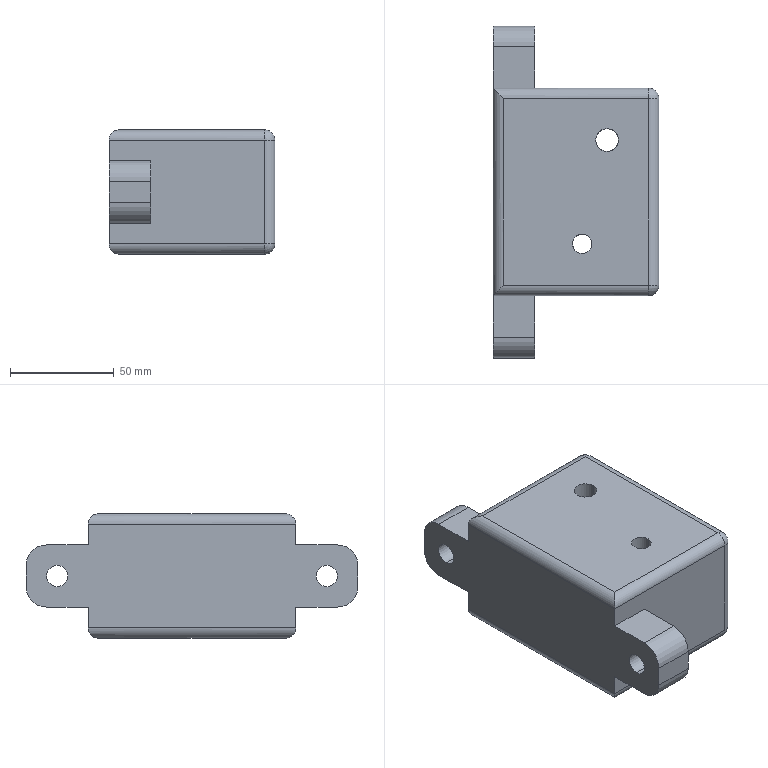Part | SolidWorks | features ICE 5, Extrusion 1, Fillet 1 | 1 solid | 58 faces | box 80 x 160 x 60 mm | volume 411118 mm3 | cylinder 30 | plane 24 | sphere 4 | commonest cylinder face diameters 10 x10 9.411 x4 10.2 x4 11 x4 20 x4 31 x4